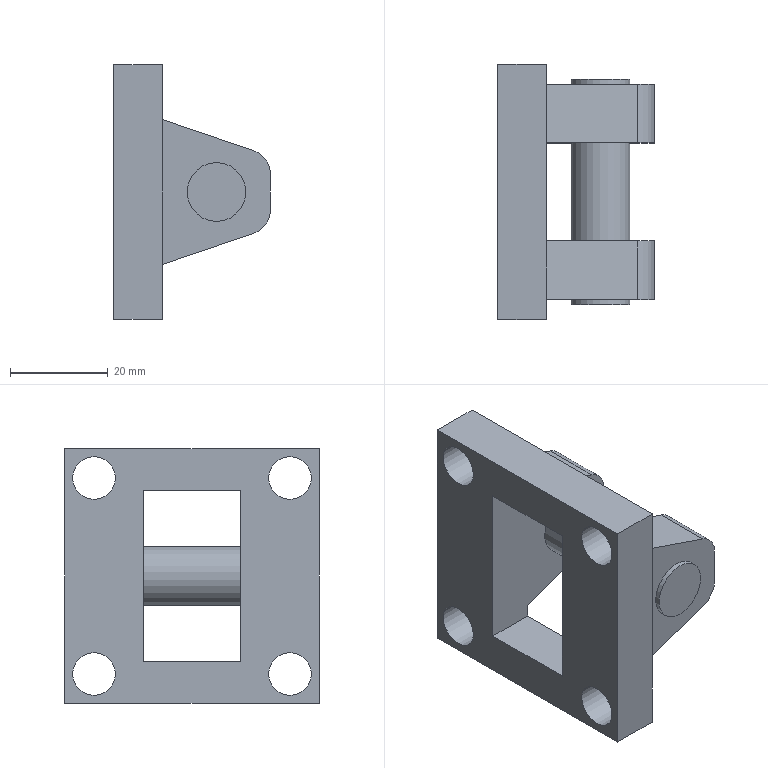Part | STEP file | 冲床-300配套压波_id670_x_t | 1 solid | 31 faces | box 32 x 52 x 52 mm | volume 31697 mm3 | plane 20 | cylinder 11 | commonest cylinder face diameters 8.7 x4 10 x4 12 x3
STEP:
#1=CARTESIAN_POINT('',(1965.,-26.,-387.));
#2=VERTEX_POINT('',#1);
#3=CARTESIAN_POINT('',(1965.,26.,-387.));
#4=VERTEX_POINT('',#3);
#5=CARTESIAN_POINT('',(1965.,-26.,-387.));
#6=DIRECTION('',(0.,1.,0.));
#7=VECTOR('',#6,1.);
#8=LINE('',#5,#7);
#9=EDGE_CURVE('',#2,#4,#8,.T.);
#10=ORIENTED_EDGE('',*,*,#9,.T.);
#11=CARTESIAN_POINT('',(1965.,26.,-335.));
#12=VERTEX_POINT('',#11);
#13=CARTESIAN_POINT('',(1965.,26.,-387.));
#14=DIRECTION('',(0.,0.,1.));
#15=VECTOR('',#14,1.);
#16=LINE('',#13,#15);
#17=EDGE_CURVE('',#4,#12,#16,.T.);
#18=ORIENTED_EDGE('',*,*,#17,.T.);
#19=CARTESIAN_POINT('',(1965.,-26.,-335.));
#20=VERTEX_POINT('',#19);
#21=CARTESIAN_POINT('',(1965.,26.,-335.));
#22=DIRECTION('',(0.,-1.,0.));
#23=VECTOR('',#22,1.);
#24=LINE('',#21,#23);
#25=EDGE_CURVE('',#12,#20,#24,.T.);
#26=ORIENTED_EDGE('',*,*,#25,.T.);
#27=CARTESIAN_POINT('',(1965.,-26.,-335.));
#28=DIRECTION('',(0.,0.,-1.));
#29=VECTOR('',#28,1.);
#30=LINE('',#27,#29);
#31=EDGE_CURVE('',#20,#2,#30,.T.);
#32=ORIENTED_EDGE('',*,*,#31,.T.);
#33=EDGE_LOOP('',(#10,#18,#26,#32));
#34=FACE_BOUND('',#33,.T.);
#35=CARTESIAN_POINT('',(1965.,-20.,-385.35));
#36=VERTEX_POINT('',#35);
#37=CARTESIAN_POINT('',(1965.,-20.,-381.));
#38=DIRECTION('',(1.,0.,0.));
#39=DIRECTION('',(0.,0.,-1.));
#40=AXIS2_PLACEMENT_3D('',#37,#38,#39);
#41=CIRCLE('',#40,4.35);
#42=EDGE_CURVE('',#36,#36,#41,.T.);
#43=ORIENTED_EDGE('',*,*,#42,.F.);
#44=EDGE_LOOP('',(#43));
#45=FACE_BOUND('',#44,.T.);
#46=CARTESIAN_POINT('',(1965.,-20.,-345.35));
#47=VERTEX_POINT('',#46);
#48=CARTESIAN_POINT('',(1965.,-20.,-341.));
#49=DIRECTION('',(1.,0.,0.));
#50=DIRECTION('',(0.,0.,-1.));
#51=AXIS2_PLACEMENT_3D('',#48,#49,#50);
#52=CIRCLE('',#51,4.35);
#53=EDGE_CURVE('',#47,#47,#52,.T.);
#54=ORIENTED_EDGE('',*,*,#53,.F.);
#55=EDGE_LOOP('',(#54));
#56=FACE_BOUND('',#55,.T.);
#57=CARTESIAN_POINT('',(1965.,20.,-385.35));
#58=VERTEX_POINT('',#57);
#59=CARTESIAN_POINT('',(1965.,20.,-381.));
#60=DIRECTION('',(1.,0.,0.));
#61=DIRECTION('',(0.,0.,-1.));
#62=AXIS2_PLACEMENT_3D('',#59,#60,#61);
#63=CIRCLE('',#62,4.35);
#64=EDGE_CURVE('',#58,#58,#63,.T.);
#65=ORIENTED_EDGE('',*,*,#64,.F.);
#66=EDGE_LOOP('',(#65));
#67=FACE_BOUND('',#66,.T.);
#68=CARTESIAN_POINT('',(1965.,20.,-345.35));
#69=VERTEX_POINT('',#68);
#70=CARTESIAN_POINT('',(1965.,20.,-341.));
#71=DIRECTION('',(1.,0.,0.));
#72=DIRECTION('',(0.,0.,-1.));
#73=AXIS2_PLACEMENT_3D('',#70,#71,#72);
#74=CIRCLE('',#73,4.35);
#75=EDGE_CURVE('',#69,#69,#74,.T.);
#76=ORIENTED_EDGE('',*,*,#75,.F.);
#77=EDGE_LOOP('',(#76));
#78=FACE_BOUND('',#77,.T.);
#79=CARTESIAN_POINT('',(1965.,10.,-343.5));
#80=VERTEX_POINT('',#79);
#81=CARTESIAN_POINT('',(1965.,10.,-346.208));
#82=VERTEX_POINT('',#81);
#83=CARTESIAN_POINT('',(1965.,10.,-343.5));
#84=DIRECTION('',(0.,0.,-1.));
#85=VECTOR('',#84,1.);
#86=LINE('',#83,#85);
#87=EDGE_CURVE('',#80,#82,#86,.T.);
#88=ORIENTED_EDGE('',*,*,#87,.T.);
#89=CARTESIAN_POINT('',(1965.,22.,-346.208));
#90=VERTEX_POINT('',#89);
#91=CARTESIAN_POINT('',(1965.,10.,-346.208));
#92=DIRECTION('',(0.,1.,0.));
#93=VECTOR('',#92,1.);
#94=LINE('',#91,#93);
#95=EDGE_CURVE('',#82,#90,#94,.T.);
#96=ORIENTED_EDGE('',*,*,#95,.T.);
#97=CARTESIAN_POINT('',(1965.,22.,-375.792));
#98=VERTEX_POINT('',#97);
#99=CARTESIAN_POINT('',(1965.,22.,-381.));
#100=DIRECTION('',(0.,0.,-1.));
#101=VECTOR('',#100,1.);
#102=LINE('',#99,#101);
#103=EDGE_CURVE('',#90,#98,#102,.T.);
#104=ORIENTED_EDGE('',*,*,#103,.T.);
#105=CARTESIAN_POINT('',(1965.,10.,-375.792));
#106=VERTEX_POINT('',#105);
#107=CARTESIAN_POINT('',(1965.,22.,-375.792));
#108=DIRECTION('',(0.,-1.,0.));
#109=VECTOR('',#108,1.);
#110=LINE('',#107,#109);
#111=EDGE_CURVE('',#98,#106,#110,.T.);
#112=ORIENTED_EDGE('',*,*,#111,.T.);
#113=CARTESIAN_POINT('',(1965.,10.,-378.5));
#114=VERTEX_POINT('',#113);
#115=CARTESIAN_POINT('',(1965.,10.,-343.5));
#116=DIRECTION('',(0.,0.,-1.));
#117=VECTOR('',#116,1.);
#118=LINE('',#115,#117);
#119=EDGE_CURVE('',#106,#114,#118,.T.);
#120=ORIENTED_EDGE('',*,*,#119,.T.);
#121=CARTESIAN_POINT('',(1965.,-10.,-378.5));
#122=VERTEX_POINT('',#121);
#123=CARTESIAN_POINT('',(1965.,10.,-378.5));
#124=DIRECTION('',(0.,-1.,0.));
#125=VECTOR('',#124,1.);
#126=LINE('',#123,#125);
#127=EDGE_CURVE('',#114,#122,#126,.T.);
#128=ORIENTED_EDGE('',*,*,#127,.T.);
#129=CARTESIAN_POINT('',(1965.,-10.,-375.792));
#130=VERTEX_POINT('',#129);
#131=CARTESIAN_POINT('',(1965.,-10.,-378.5));
#132=DIRECTION('',(0.,0.,1.));
#133=VECTOR('',#132,1.);
#134=LINE('',#131,#133);
#135=EDGE_CURVE('',#122,#130,#134,.T.);
#136=ORIENTED_EDGE('',*,*,#135,.T.);
#137=CARTESIAN_POINT('',(1965.,-22.,-375.792));
#138=VERTEX_POINT('',#137);
#139=CARTESIAN_POINT('',(1965.,-20.,-375.792));
#140=DIRECTION('',(0.,-1.,0.));
#141=VECTOR('',#140,1.);
#142=LINE('',#139,#141);
#143=EDGE_CURVE('',#130,#138,#142,.T.);
#144=ORIENTED_EDGE('',*,*,#143,.T.);
#145=CARTESIAN_POINT('',(1965.,-22.,-346.208));
#146=VERTEX_POINT('',#145);
#147=CARTESIAN_POINT('',(1965.,-22.,-381.));
#148=DIRECTION('',(0.,0.,1.));
#149=VECTOR('',#148,1.);
#150=LINE('',#147,#149);
#151=EDGE_CURVE('',#138,#146,#150,.T.);
#152=ORIENTED_EDGE('',*,*,#151,.T.);
#153=CARTESIAN_POINT('',(1965.,-10.,-346.208));
#154=VERTEX_POINT('',#153);
#155=CARTESIAN_POINT('',(1965.,-20.,-346.208));
#156=DIRECTION('',(0.,1.,0.));
#157=VECTOR('',#156,1.);
#158=LINE('',#155,#157);
#159=EDGE_CURVE('',#146,#154,#158,.T.);
#160=ORIENTED_EDGE('',*,*,#159,.T.);
#161=CARTESIAN_POINT('',(1965.,-10.,-343.5));
#162=VERTEX_POINT('',#161);
#163=CARTESIAN_POINT('',(1965.,-10.,-378.5));
#164=DIRECTION('',(0.,0.,1.));
#165=VECTOR('',#164,1.);
#166=LINE('',#163,#165);
#167=EDGE_CURVE('',#154,#162,#166,.T.);
#168=ORIENTED_EDGE('',*,*,#167,.T.);
#169=CARTESIAN_POINT('',(1965.,-10.,-343.5));
#170=DIRECTION('',(0.,1.,0.));
#171=VECTOR('',#170,1.);
#172=LINE('',#169,#171);
#173=EDGE_CURVE('',#162,#80,#172,.T.);
#174=ORIENTED_EDGE('',*,*,#173,.T.);
#175=EDGE_LOOP('',(#88,#96,#104,#112,#120,#128,#136,#144,#152,#160,#168,#174));
#176=FACE_BOUND('',#175,.T.);
#177=CARTESIAN_POINT('',(1965.,-20.,-381.));
#178=DIRECTION('',(1.,0.,0.));
#179=DIRECTION('',(0.,0.,-1.));
#180=AXIS2_PLACEMENT_3D('',#177,#178,#179);
#181=PLANE('',#180);
#182=ADVANCED_FACE('',(#34,#45,#56,#67,#78,#176),#181,.T.);
#183=CARTESIAN_POINT('',(1976.,-10.,-355.));
#184=VERTEX_POINT('',#183);
#185=CARTESIAN_POINT('',(1976.,-10.,-361.));
#186=DIRECTION('',(0.,1.,0.));
#187=DIRECTION('',(0.,0.,1.));
#188=AXIS2_PLACEMENT_3D('',#185,#186,#187);
#189=CIRCLE('',#188,6.);
#190=EDGE_CURVE('',#184,#184,#189,.T.);
#191=ORIENTED_EDGE('',*,*,#190,.F.);
#192=EDGE_LOOP('',(#191));
#193=FACE_BOUND('',#192,.T.);
#194=CARTESIAN_POINT('',(1983.613,-10.,-352.554));
#195=VERTEX_POINT('',#194);
#196=CARTESIAN_POINT('',(1965.903,-10.,-346.516));
#197=DIRECTION('',(0.9465,0.,-0.3227));
#198=VECTOR('',#197,1.);
#199=LINE('',#196,#198);
#200=EDGE_CURVE('',#154,#195,#199,.T.);
#201=ORIENTED_EDGE('',*,*,#200,.T.);
#202=CARTESIAN_POINT('',(1987.,-10.,-357.286));
#203=VERTEX_POINT('',#202);
#204=CARTESIAN_POINT('',(1982.,-10.,-357.286));
#205=DIRECTION('',(0.,1.,0.));
#206=DIRECTION('',(0.,0.,1.));
#207=AXIS2_PLACEMENT_3D('',#204,#205,#206);
#208=CIRCLE('',#207,5.);
#209=EDGE_CURVE('',#195,#203,#208,.T.);
#210=ORIENTED_EDGE('',*,*,#209,.T.);
#211=CARTESIAN_POINT('',(1987.,-10.,-364.714));
#212=VERTEX_POINT('',#211);
#213=CARTESIAN_POINT('',(1987.,-10.,-346.208));
#214=DIRECTION('',(0.,0.,-1.));
#215=VECTOR('',#214,1.);
#216=LINE('',#213,#215);
#217=EDGE_CURVE('',#203,#212,#216,.T.);
#218=ORIENTED_EDGE('',*,*,#217,.T.);
#219=CARTESIAN_POINT('',(1983.613,-10.,-369.446));
#220=VERTEX_POINT('',#219);
#221=CARTESIAN_POINT('',(1982.,-10.,-364.714));
#222=DIRECTION('',(0.,1.,0.));
#223=DIRECTION('',(0.,0.,1.));
#224=AXIS2_PLACEMENT_3D('',#221,#222,#223);
#225=CIRCLE('',#224,5.);
#226=EDGE_CURVE('',#212,#220,#225,.T.);
#227=ORIENTED_EDGE('',*,*,#226,.T.);
#228=CARTESIAN_POINT('',(1955.214,-10.,-379.128));
#229=DIRECTION('',(-0.9465,0.,-0.3227));
#230=VECTOR('',#229,1.);
#231=LINE('',#228,#230);
#232=EDGE_CURVE('',#220,#130,#231,.T.);
#233=ORIENTED_EDGE('',*,*,#232,.T.);
#234=ORIENTED_EDGE('',*,*,#135,.F.);
#235=CARTESIAN_POINT('',(1955.,-10.,-378.5));
#236=VERTEX_POINT('',#235);
#237=CARTESIAN_POINT('',(1955.,-10.,-378.5));
#238=DIRECTION('',(1.,0.,0.));
#239=VECTOR('',#238,1.);
#240=LINE('',#237,#239);
#241=EDGE_CURVE('',#236,#122,#240,.T.);
#242=ORIENTED_EDGE('',*,*,#241,.F.);
#243=CARTESIAN_POINT('',(1955.,-10.,-343.5));
#244=VERTEX_POINT('',#243);
#245=CARTESIAN_POINT('',(1955.,-10.,-378.5));
#246=DIRECTION('',(0.,0.,1.));
#247=VECTOR('',#246,1.);
#248=LINE('',#245,#247);
#249=EDGE_CURVE('',#236,#244,#248,.T.);
#250=ORIENTED_EDGE('',*,*,#249,.T.);
#251=CARTESIAN_POINT('',(1955.,-10.,-343.5));
#252=DIRECTION('',(1.,0.,0.));
#253=VECTOR('',#252,1.);
#254=LINE('',#251,#253);
#255=EDGE_CURVE('',#244,#162,#254,.T.);
#256=ORIENTED_EDGE('',*,*,#255,.T.);
#257=ORIENTED_EDGE('',*,*,#167,.F.);
#258=EDGE_LOOP('',(#201,#210,#218,#227,#233,#234,#242,#250,#256,#257));
#259=FACE_BOUND('',#258,.T.);
#260=CARTESIAN_POINT('',(1955.,-10.,-378.5));
#261=DIRECTION('',(0.,1.,0.));
#262=DIRECTION('',(0.,0.,1.));
#263=AXIS2_PLACEMENT_3D('',#260,#261,#262);
#264=PLANE('',#263);
#265=ADVANCED_FACE('',(#193,#259),#264,.T.);
#266=ORIENTED_EDGE('',*,*,#173,.F.);
#267=ORIENTED_EDGE('',*,*,#255,.F.);
#268=CARTESIAN_POINT('',(1955.,10.,-343.5));
#269=VERTEX_POINT('',#268);
#270=CARTESIAN_POINT('',(1955.,-10.,-343.5));
#271=DIRECTION('',(0.,1.,0.));
#272=VECTOR('',#271,1.);
#273=LINE('',#270,#272);
#274=EDGE_CURVE('',#244,#269,#273,.T.);
#275=ORIENTED_EDGE('',*,*,#274,.T.);
#276=CARTESIAN_POINT('',(1955.,10.,-343.5));
#277=DIRECTION('',(1.,0.,0.));
#278=VECTOR('',#277,1.);
#279=LINE('',#276,#278);
#280=EDGE_CURVE('',#269,#80,#279,.T.);
#281=ORIENTED_EDGE('',*,*,#280,.T.);
#282=EDGE_LOOP('',(#266,#267,#275,#281));
#283=FACE_OUTER_BOUND('',#282,.T.);
#284=CARTESIAN_POINT('',(1955.,-10.,-343.5));
#285=DIRECTION('',(0.,0.,-1.));
#286=DIRECTION('',(0.,1.,0.));
#287=AXIS2_PLACEMENT_3D('',#284,#285,#286);
#288=PLANE('',#287);
#289=ADVANCED_FACE('',(#283),#288,.T.);
#290=CARTESIAN_POINT('',(1976.,10.,-367.));
#291=VERTEX_POINT('',#290);
#292=CARTESIAN_POINT('',(1976.,10.,-361.));
#293=DIRECTION('',(0.,-1.,0.));
#294=DIRECTION('',(0.,0.,-1.));
#295=AXIS2_PLACEMENT_3D('',#292,#293,#294);
#296=CIRCLE('',#295,6.);
#297=EDGE_CURVE('',#291,#291,#296,.T.);
#298=ORIENTED_EDGE('',*,*,#297,.F.);
#299=EDGE_LOOP('',(#298));
#300=FACE_BOUND('',#299,.T.);
#301=CARTESIAN_POINT('',(1983.613,10.,-369.446));
#302=VERTEX_POINT('',#301);
#303=CARTESIAN_POINT('',(1965.,10.,-375.792));
#304=DIRECTION('',(0.9465,0.,0.3227));
#305=VECTOR('',#304,1.);
#306=LINE('',#303,#305);
#307=EDGE_CURVE('',#106,#302,#306,.T.);
#308=ORIENTED_EDGE('',*,*,#307,.T.);
#309=CARTESIAN_POINT('',(1987.,10.,-364.714));
#310=VERTEX_POINT('',#309);
#311=CARTESIAN_POINT('',(1982.,10.,-364.714));
#312=DIRECTION('',(0.,-1.,0.));
#313=DIRECTION('',(0.,0.,-1.));
#314=AXIS2_PLACEMENT_3D('',#311,#312,#313);
#315=CIRCLE('',#314,5.);
#316=EDGE_CURVE('',#302,#310,#315,.T.);
#317=ORIENTED_EDGE('',*,*,#316,.T.);
#318=CARTESIAN_POINT('',(1987.,10.,-357.286));
#319=VERTEX_POINT('',#318);
#320=CARTESIAN_POINT('',(1987.,10.,-375.792));
#321=DIRECTION('',(0.,0.,1.));
#322=VECTOR('',#321,1.);
#323=LINE('',#320,#322);
#324=EDGE_CURVE('',#310,#319,#323,.T.);
#325=ORIENTED_EDGE('',*,*,#324,.T.);
#326=CARTESIAN_POINT('',(1983.613,10.,-352.554));
#327=VERTEX_POINT('',#326);
#328=CARTESIAN_POINT('',(1982.,10.,-357.286));
#329=DIRECTION('',(0.,-1.,0.));
#330=DIRECTION('',(0.,0.,-1.));
#331=AXIS2_PLACEMENT_3D('',#328,#329,#330);
#332=CIRCLE('',#331,5.);
#333=EDGE_CURVE('',#319,#327,#332,.T.);
#334=ORIENTED_EDGE('',*,*,#333,.T.);
#335=CARTESIAN_POINT('',(1965.,10.,-346.208));
#336=DIRECTION('',(-0.9465,0.,0.3227));
#337=VECTOR('',#336,1.);
#338=LINE('',#335,#337);
#339=EDGE_CURVE('',#327,#82,#338,.T.);
#340=ORIENTED_EDGE('',*,*,#339,.T.);
#341=ORIENTED_EDGE('',*,*,#87,.F.);
#342=ORIENTED_EDGE('',*,*,#280,.F.);
#343=CARTESIAN_POINT('',(1955.,10.,-378.5));
#344=VERTEX_POINT('',#343);
#345=CARTESIAN_POINT('',(1955.,10.,-343.5));
#346=DIRECTION('',(0.,0.,-1.));
#347=VECTOR('',#346,1.);
#348=LINE('',#345,#347);
#349=EDGE_CURVE('',#269,#344,#348,.T.);
#350=ORIENTED_EDGE('',*,*,#349,.T.);
#351=CARTESIAN_POINT('',(1955.,10.,-378.5));
#352=DIRECTION('',(1.,0.,0.));
#353=VECTOR('',#352,1.);
#354=LINE('',#351,#353);
#355=EDGE_CURVE('',#344,#114,#354,.T.);
#356=ORIENTED_EDGE('',*,*,#355,.T.);
#357=ORIENTED_EDGE('',*,*,#119,.F.);
#358=EDGE_LOOP('',(#308,#317,#325,#334,#340,#341,#342,#350,#356,#357));
#359=FACE_BOUND('',#358,.T.);
#360=CARTESIAN_POINT('',(1955.,10.,-343.5));
#361=DIRECTION('',(0.,-1.,0.));
#362=DIRECTION('',(0.,0.,-1.));
#363=AXIS2_PLACEMENT_3D('',#360,#361,#362);
#364=PLANE('',#363);
#365=ADVANCED_FACE('',(#300,#359),#364,.T.);
#366=ORIENTED_EDGE('',*,*,#9,.F.);
#367=CARTESIAN_POINT('',(1955.,-26.,-387.));
#368=VERTEX_POINT('',#367);
#369=CARTESIAN_POINT('',(1955.,-26.,-387.));
#370=DIRECTION('',(1.,0.,0.));
#371=VECTOR('',#370,1.);
#372=LINE('',#369,#371);
#373=EDGE_CURVE('',#368,#2,#372,.T.);
#374=ORIENTED_EDGE('',*,*,#373,.F.);
#375=CARTESIAN_POINT('',(1955.,26.,-387.));
#376=VERTEX_POINT('',#375);
#377=CARTESIAN_POINT('',(1955.,-26.,-387.));
#378=DIRECTION('',(0.,1.,0.));
#379=VECTOR('',#378,1.);
#380=LINE('',#377,#379);
#381=EDGE_CURVE('',#368,#376,#380,.T.);
#382=ORIENTED_EDGE('',*,*,#381,.T.);
#383=CARTESIAN_POINT('',(1955.,26.,-387.));
#384=DIRECTION('',(1.,0.,0.));
#385=VECTOR('',#384,1.);
#386=LINE('',#383,#385);
#387=EDGE_CURVE('',#376,#4,#386,.T.);
#388=ORIENTED_EDGE('',*,*,#387,.T.);
#389=EDGE_LOOP('',(#366,#374,#382,#388));
#390=FACE_OUTER_BOUND('',#389,.T.);
#391=CARTESIAN_POINT('',(1955.,-26.,-387.));
#392=DIRECTION('',(0.,0.,-1.));
#393=DIRECTION('',(-1.,0.,0.));
#394=AXIS2_PLACEMENT_3D('',#391,#392,#393);
#395=PLANE('',#394);
#396=ADVANCED_FACE('',(#390),#395,.T.);
#397=ORIENTED_EDGE('',*,*,#17,.F.);
#398=ORIENTED_EDGE('',*,*,#387,.F.);
#399=CARTESIAN_POINT('',(1955.,26.,-335.));
#400=VERTEX_POINT('',#399);
#401=CARTESIAN_POINT('',(1955.,26.,-387.));
#402=DIRECTION('',(0.,0.,1.));
#403=VECTOR('',#402,1.);
#404=LINE('',#401,#403);
#405=EDGE_CURVE('',#376,#400,#404,.T.);
#406=ORIENTED_EDGE('',*,*,#405,.T.);
#407=CARTESIAN_POINT('',(1955.,26.,-335.));
#408=DIRECTION('',(1.,0.,0.));
#409=VECTOR('',#408,1.);
#410=LINE('',#407,#409);
#411=EDGE_CURVE('',#400,#12,#410,.T.);
#412=ORIENTED_EDGE('',*,*,#411,.T.);
#413=EDGE_LOOP('',(#397,#398,#406,#412));
#414=FACE_OUTER_BOUND('',#413,.T.);
#415=CARTESIAN_POINT('',(1955.,26.,-387.));
#416=DIRECTION('',(0.,1.,0.));
#417=DIRECTION('',(0.,0.,1.));
#418=AXIS2_PLACEMENT_3D('',#415,#416,#417);
#419=PLANE('',#418);
#420=ADVANCED_FACE('',(#414),#419,.T.);
#421=ORIENTED_EDGE('',*,*,#25,.F.);
#422=ORIENTED_EDGE('',*,*,#411,.F.);
#423=CARTESIAN_POINT('',(1955.,-26.,-335.));
#424=VERTEX_POINT('',#423);
#425=CARTESIAN_POINT('',(1955.,26.,-335.));
#426=DIRECTION('',(0.,-1.,0.));
#427=VECTOR('',#426,1.);
#428=LINE('',#425,#427);
#429=EDGE_CURVE('',#400,#424,#428,.T.);
#430=ORIENTED_EDGE('',*,*,#429,.T.);
#431=CARTESIAN_POINT('',(1955.,-26.,-335.));
#432=DIRECTION('',(1.,0.,0.));
#433=VECTOR('',#432,1.);
#434=LINE('',#431,#433);
#435=EDGE_CURVE('',#424,#20,#434,.T.);
#436=ORIENTED_EDGE('',*,*,#435,.T.);
#437=EDGE_LOOP('',(#421,#422,#430,#436));
#438=FACE_OUTER_BOUND('',#437,.T.);
#439=CARTESIAN_POINT('',(1955.,26.,-335.));
#440=DIRECTION('',(0.,0.,1.));
#441=DIRECTION('',(1.,0.,0.));
#442=AXIS2_PLACEMENT_3D('',#439,#440,#441);
#443=PLANE('',#442);
#444=ADVANCED_FACE('',(#438),#443,.T.);
#445=CARTESIAN_POINT('',(1955.,20.,-345.35));
#446=VERTEX_POINT('',#445);
#447=CARTESIAN_POINT('',(1955.,20.,-341.));
#448=DIRECTION('',(1.,0.,0.));
#449=DIRECTION('',(0.,0.,-1.));
#450=AXIS2_PLACEMENT_3D('',#447,#448,#449);
#451=CIRCLE('',#450,4.35);
#452=EDGE_CURVE('',#446,#446,#451,.T.);
#453=ORIENTED_EDGE('',*,*,#452,.F.);
#454=EDGE_LOOP('',(#453));
#455=FACE_BOUND('',#454,.T.);
#456=ORIENTED_EDGE('',*,*,#75,.T.);
#457=EDGE_LOOP('',(#456));
#458=FACE_BOUND('',#457,.T.);
#459=CARTESIAN_POINT('',(1955.,20.,-341.));
#460=DIRECTION('',(1.,0.,0.));
#461=DIRECTION('',(0.,0.,-1.));
#462=AXIS2_PLACEMENT_3D('',#459,#460,#461);
#463=CYLINDRICAL_SURFACE('',#462,4.35);
#464=ADVANCED_FACE('',(#455,#458),#463,.F.);
#465=CARTESIAN_POINT('',(1955.,20.,-385.35));
#466=VERTEX_POINT('',#465);
#467=CARTESIAN_POINT('',(1955.,20.,-381.));
#468=DIRECTION('',(1.,0.,0.));
#469=DIRECTION('',(0.,0.,-1.));
#470=AXIS2_PLACEMENT_3D('',#467,#468,#469);
#471=CIRCLE('',#470,4.35);
#472=EDGE_CURVE('',#466,#466,#471,.T.);
#473=ORIENTED_EDGE('',*,*,#472,.F.);
#474=EDGE_LOOP('',(#473));
#475=FACE_BOUND('',#474,.T.);
#476=ORIENTED_EDGE('',*,*,#64,.T.);
#477=EDGE_LOOP('',(#476));
#478=FACE_BOUND('',#477,.T.);
#479=CARTESIAN_POINT('',(1955.,20.,-381.));
#480=DIRECTION('',(1.,0.,0.));
#481=DIRECTION('',(0.,0.,-1.));
#482=AXIS2_PLACEMENT_3D('',#479,#480,#481);
#483=CYLINDRICAL_SURFACE('',#482,4.35);
#484=ADVANCED_FACE('',(#475,#478),#483,.F.);
#485=CARTESIAN_POINT('',(1955.,-20.,-345.35));
#486=VERTEX_POINT('',#485);
#487=CARTESIAN_POINT('',(1955.,-20.,-341.));
#488=DIRECTION('',(1.,0.,0.));
#489=DIRECTION('',(0.,0.,-1.));
#490=AXIS2_PLACEMENT_3D('',#487,#488,#489);
#491=CIRCLE('',#490,4.35);
#492=EDGE_CURVE('',#486,#486,#491,.T.);
#493=ORIENTED_EDGE('',*,*,#492,.F.);
#494=EDGE_LOOP('',(#493));
#495=FACE_BOUND('',#494,.T.);
#496=ORIENTED_EDGE('',*,*,#53,.T.);
#497=EDGE_LOOP('',(#496));
#498=FACE_BOUND('',#497,.T.);
#499=CARTESIAN_POINT('',(1955.,-20.,-341.));
#500=DIRECTION('',(1.,0.,0.));
#501=DIRECTION('',(0.,0.,-1.));
#502=AXIS2_PLACEMENT_3D('',#499,#500,#501);
#503=CYLINDRICAL_SURFACE('',#502,4.35);
#504=ADVANCED_FACE('',(#495,#498),#503,.F.);
#505=CARTESIAN_POINT('',(1955.,-20.,-385.35));
#506=VERTEX_POINT('',#505);
#507=CARTESIAN_POINT('',(1955.,-20.,-381.));
#508=DIRECTION('',(1.,0.,0.));
#509=DIRECTION('',(0.,0.,-1.));
#510=AXIS2_PLACEMENT_3D('',#507,#508,#509);
#511=CIRCLE('',#510,4.35);
#512=EDGE_CURVE('',#506,#506,#511,.T.);
#513=ORIENTED_EDGE('',*,*,#512,.F.);
#514=EDGE_LOOP('',(#513));
#515=FACE_BOUND('',#514,.T.);
#516=ORIENTED_EDGE('',*,*,#42,.T.);
#517=EDGE_LOOP('',(#516));
#518=FACE_BOUND('',#517,.T.);
#519=CARTESIAN_POINT('',(1955.,-20.,-381.));
#520=DIRECTION('',(1.,0.,0.));
#521=DIRECTION('',(0.,0.,-1.));
#522=AXIS2_PLACEMENT_3D('',#519,#520,#521);
#523=CYLINDRICAL_SURFACE('',#522,4.35);
#524=ADVANCED_FACE('',(#515,#518),#523,.F.);
#525=ORIENTED_EDGE('',*,*,#31,.F.);
#526=ORIENTED_EDGE('',*,*,#435,.F.);
#527=CARTESIAN_POINT('',(1955.,-26.,-335.));
#528=DIRECTION('',(0.,0.,-1.));
#529=VECTOR('',#528,1.);
#530=LINE('',#527,#529);
#531=EDGE_CURVE('',#424,#368,#530,.T.);
#532=ORIENTED_EDGE('',*,*,#531,.T.);
#533=ORIENTED_EDGE('',*,*,#373,.T.);
#534=EDGE_LOOP('',(#525,#526,#532,#533));
#535=FACE_OUTER_BOUND('',#534,.T.);
#536=CARTESIAN_POINT('',(1955.,-26.,-335.));
#537=DIRECTION('',(0.,-1.,0.));
#538=DIRECTION('',(0.,0.,-1.));
#539=AXIS2_PLACEMENT_3D('',#536,#537,#538);
#540=PLANE('',#539);
#541=ADVANCED_FACE('',(#535),#540,.T.);
#542=ORIENTED_EDGE('',*,*,#127,.F.);
#543=ORIENTED_EDGE('',*,*,#355,.F.);
#544=CARTESIAN_POINT('',(1955.,10.,-378.5));
#545=DIRECTION('',(0.,-1.,0.));
#546=VECTOR('',#545,1.);
#547=LINE('',#544,#546);
#548=EDGE_CURVE('',#344,#236,#547,.T.);
#549=ORIENTED_EDGE('',*,*,#548,.T.);
#550=ORIENTED_EDGE('',*,*,#241,.T.);
#551=EDGE_LOOP('',(#542,#543,#549,#550));
#552=FACE_OUTER_BOUND('',#551,.T.);
#553=CARTESIAN_POINT('',(1955.,10.,-378.5));
#554=DIRECTION('',(0.,0.,1.));
#555=DIRECTION('',(0.,-1.,0.));
#556=AXIS2_PLACEMENT_3D('',#553,#554,#555);
#557=PLANE('',#556);
#558=ADVANCED_FACE('',(#552),#557,.T.);
#559=ORIENTED_EDGE('',*,*,#548,.F.);
#560=ORIENTED_EDGE('',*,*,#349,.F.);
#561=ORIENTED_EDGE('',*,*,#274,.F.);
#562=ORIENTED_EDGE('',*,*,#249,.F.);
#563=EDGE_LOOP('',(#559,#560,#561,#562));
#564=FACE_BOUND('',#563,.T.);
#565=ORIENTED_EDGE('',*,*,#381,.F.);
#566=ORIENTED_EDGE('',*,*,#531,.F.);
#567=ORIENTED_EDGE('',*,*,#429,.F.);
#568=ORIENTED_EDGE('',*,*,#405,.F.);
#569=EDGE_LOOP('',(#565,#566,#567,#568));
#570=FACE_BOUND('',#569,.T.);
#571=ORIENTED_EDGE('',*,*,#512,.T.);
#572=EDGE_LOOP('',(#571));
#573=FACE_BOUND('',#572,.T.);
#574=ORIENTED_EDGE('',*,*,#492,.T.);
#575=EDGE_LOOP('',(#574));
#576=FACE_BOUND('',#575,.T.);
#577=ORIENTED_EDGE('',*,*,#472,.T.);
#578=EDGE_LOOP('',(#577));
#579=FACE_BOUND('',#578,.T.);
#580=ORIENTED_EDGE('',*,*,#452,.T.);
#581=EDGE_LOOP('',(#580));
#582=FACE_BOUND('',#581,.T.);
#583=CARTESIAN_POINT('',(1955.,-20.,-381.));
#584=DIRECTION('',(1.,0.,0.));
#585=DIRECTION('',(0.,0.,-1.));
#586=AXIS2_PLACEMENT_3D('',#583,#584,#585);
#587=PLANE('',#586);
#588=ADVANCED_FACE('',(#564,#570,#573,#576,#579,#582),#587,.F.);
#589=CARTESIAN_POINT('',(1976.,-22.,-355.));
#590=VERTEX_POINT('',#589);
#591=CARTESIAN_POINT('',(1976.,-22.,-361.));
#592=DIRECTION('',(0.,1.,0.));
#593=DIRECTION('',(0.,0.,1.));
#594=AXIS2_PLACEMENT_3D('',#591,#592,#593);
#595=CIRCLE('',#594,6.);
#596=EDGE_CURVE('',#590,#590,#595,.T.);
#597=ORIENTED_EDGE('',*,*,#596,.T.);
#598=EDGE_LOOP('',(#597));
#599=FACE_BOUND('',#598,.T.);
#600=CARTESIAN_POINT('',(1987.,-22.,-364.714));
#601=VERTEX_POINT('',#600);
#602=CARTESIAN_POINT('',(1987.,-22.,-357.286));
#603=VERTEX_POINT('',#602);
#604=CARTESIAN_POINT('',(1987.,-22.,-375.792));
#605=DIRECTION('',(0.,0.,1.));
#606=VECTOR('',#605,1.);
#607=LINE('',#604,#606);
#608=EDGE_CURVE('',#601,#603,#607,.T.);
#609=ORIENTED_EDGE('',*,*,#608,.T.);
#610=CARTESIAN_POINT('',(1983.613,-22.,-352.554));
#611=VERTEX_POINT('',#610);
#612=CARTESIAN_POINT('',(1982.,-22.,-357.286));
#613=DIRECTION('',(0.,-1.,0.));
#614=DIRECTION('',(0.,0.,1.));
#615=AXIS2_PLACEMENT_3D('',#612,#613,#614);
#616=CIRCLE('',#615,5.);
#617=EDGE_CURVE('',#603,#611,#616,.T.);
#618=ORIENTED_EDGE('',*,*,#617,.T.);
#619=CARTESIAN_POINT('',(1965.076,-22.,-346.234));
#620=DIRECTION('',(-0.9465,0.,0.3227));
#621=VECTOR('',#620,1.);
#622=LINE('',#619,#621);
#623=EDGE_CURVE('',#611,#146,#622,.T.);
#624=ORIENTED_EDGE('',*,*,#623,.T.);
#625=ORIENTED_EDGE('',*,*,#151,.F.);
#626=CARTESIAN_POINT('',(1983.613,-22.,-369.446));
#627=VERTEX_POINT('',#626);
#628=CARTESIAN_POINT('',(1956.041,-22.,-378.846));
#629=DIRECTION('',(0.9465,0.,0.3227));
#630=VECTOR('',#629,1.);
#631=LINE('',#628,#630);
#632=EDGE_CURVE('',#138,#627,#631,.T.);
#633=ORIENTED_EDGE('',*,*,#632,.T.);
#634=CARTESIAN_POINT('',(1982.,-22.,-364.714));
#635=DIRECTION('',(0.,-1.,0.));
#636=DIRECTION('',(0.,0.,1.));
#637=AXIS2_PLACEMENT_3D('',#634,#635,#636);
#638=CIRCLE('',#637,5.);
#639=EDGE_CURVE('',#627,#601,#638,.T.);
#640=ORIENTED_EDGE('',*,*,#639,.T.);
#641=EDGE_LOOP('',(#609,#618,#624,#625,#633,#640));
#642=FACE_BOUND('',#641,.T.);
#643=CARTESIAN_POINT('',(1955.,-22.,-375.792));
#644=DIRECTION('',(0.,1.,0.));
#645=DIRECTION('',(0.,0.,1.));
#646=AXIS2_PLACEMENT_3D('',#643,#644,#645);
#647=PLANE('',#646);
#648=ADVANCED_FACE('',(#599,#642),#647,.F.);
#649=ORIENTED_EDGE('',*,*,#217,.F.);
#650=CARTESIAN_POINT('',(1987.,-22.,-357.286));
#651=DIRECTION('',(0.,-1.,0.));
#652=VECTOR('',#651,1.);
#653=LINE('',#650,#652);
#654=EDGE_CURVE('',#203,#603,#653,.T.);
#655=ORIENTED_EDGE('',*,*,#654,.T.);
#656=ORIENTED_EDGE('',*,*,#608,.F.);
#657=CARTESIAN_POINT('',(1987.,-10.,-364.714));
#658=DIRECTION('',(0.,1.,0.));
#659=VECTOR('',#658,1.);
#660=LINE('',#657,#659);
#661=EDGE_CURVE('',#601,#212,#660,.T.);
#662=ORIENTED_EDGE('',*,*,#661,.T.);
#663=EDGE_LOOP('',(#649,#655,#656,#662));
#664=FACE_OUTER_BOUND('',#663,.T.);
#665=CARTESIAN_POINT('',(1987.,360.96,3.519));
#666=DIRECTION('',(-1.,0.,0.));
#667=DIRECTION('',(0.,0.,1.));
#668=AXIS2_PLACEMENT_3D('',#665,#666,#667);
#669=PLANE('',#668);
#670=ADVANCED_FACE('',(#664),#669,.F.);
#671=ORIENTED_EDGE('',*,*,#623,.F.);
#672=CARTESIAN_POINT('',(1983.613,360.96,-352.554));
#673=DIRECTION('',(0.,1.,0.));
#674=VECTOR('',#673,1.);
#675=LINE('',#672,#674);
#676=EDGE_CURVE('',#611,#195,#675,.T.);
#677=ORIENTED_EDGE('',*,*,#676,.T.);
#678=ORIENTED_EDGE('',*,*,#200,.F.);
#679=ORIENTED_EDGE('',*,*,#159,.F.);
#680=EDGE_LOOP('',(#671,#677,#678,#679));
#681=FACE_OUTER_BOUND('',#680,.T.);
#682=CARTESIAN_POINT('',(1965.,10.,-346.208));
#683=DIRECTION('',(-0.3227,0.,-0.9465));
#684=DIRECTION('',(0.,1.,0.));
#685=AXIS2_PLACEMENT_3D('',#682,#683,#684);
#686=PLANE('',#685);
#687=ADVANCED_FACE('',(#681),#686,.F.);
#688=ORIENTED_EDGE('',*,*,#232,.F.);
#689=CARTESIAN_POINT('',(1983.613,360.96,-369.446));
#690=DIRECTION('',(0.,-1.,0.));
#691=VECTOR('',#690,1.);
#692=LINE('',#689,#691);
#693=EDGE_CURVE('',#220,#627,#692,.T.);
#694=ORIENTED_EDGE('',*,*,#693,.T.);
#695=ORIENTED_EDGE('',*,*,#632,.F.);
#696=ORIENTED_EDGE('',*,*,#143,.F.);
#697=EDGE_LOOP('',(#688,#694,#695,#696));
#698=FACE_OUTER_BOUND('',#697,.T.);
#699=CARTESIAN_POINT('',(1965.,22.,-375.792));
#700=DIRECTION('',(-0.3227,0.,0.9465));
#701=DIRECTION('',(0.,-1.,0.));
#702=AXIS2_PLACEMENT_3D('',#699,#700,#701);
#703=PLANE('',#702);
#704=ADVANCED_FACE('',(#698),#703,.F.);
#705=CARTESIAN_POINT('',(1976.,22.,-367.));
#706=VERTEX_POINT('',#705);
#707=CARTESIAN_POINT('',(1976.,22.,-361.));
#708=DIRECTION('',(0.,-1.,0.));
#709=DIRECTION('',(0.,0.,-1.));
#710=AXIS2_PLACEMENT_3D('',#707,#708,#709);
#711=CIRCLE('',#710,6.);
#712=EDGE_CURVE('',#706,#706,#711,.T.);
#713=ORIENTED_EDGE('',*,*,#712,.T.);
#714=EDGE_LOOP('',(#713));
#715=FACE_BOUND('',#714,.T.);
#716=CARTESIAN_POINT('',(1987.,22.,-357.286));
#717=VERTEX_POINT('',#716);
#718=CARTESIAN_POINT('',(1987.,22.,-364.714));
#719=VERTEX_POINT('',#718);
#720=CARTESIAN_POINT('',(1987.,22.,-346.208));
#721=DIRECTION('',(0.,0.,-1.));
#722=VECTOR('',#721,1.);
#723=LINE('',#720,#722);
#724=EDGE_CURVE('',#717,#719,#723,.T.);
#725=ORIENTED_EDGE('',*,*,#724,.T.);
#726=CARTESIAN_POINT('',(1983.613,22.,-369.446));
#727=VERTEX_POINT('',#726);
#728=CARTESIAN_POINT('',(1982.,22.,-364.714));
#729=DIRECTION('',(0.,1.,0.));
#730=DIRECTION('',(0.,0.,-1.));
#731=AXIS2_PLACEMENT_3D('',#728,#729,#730);
#732=CIRCLE('',#731,5.);
#733=EDGE_CURVE('',#719,#727,#732,.T.);
#734=ORIENTED_EDGE('',*,*,#733,.T.);
#735=CARTESIAN_POINT('',(1965.,22.,-375.792));
#736=DIRECTION('',(-0.9465,0.,-0.3227));
#737=VECTOR('',#736,1.);
#738=LINE('',#735,#737);
#739=EDGE_CURVE('',#727,#98,#738,.T.);
#740=ORIENTED_EDGE('',*,*,#739,.T.);
#741=ORIENTED_EDGE('',*,*,#103,.F.);
#742=CARTESIAN_POINT('',(1983.613,22.,-352.554));
#743=VERTEX_POINT('',#742);
#744=CARTESIAN_POINT('',(1965.,22.,-346.208));
#745=DIRECTION('',(0.9465,0.,-0.3227));
#746=VECTOR('',#745,1.);
#747=LINE('',#744,#746);
#748=EDGE_CURVE('',#90,#743,#747,.T.);
#749=ORIENTED_EDGE('',*,*,#748,.T.);
#750=CARTESIAN_POINT('',(1982.,22.,-357.286));
#751=DIRECTION('',(0.,1.,0.));
#752=DIRECTION('',(0.,0.,-1.));
#753=AXIS2_PLACEMENT_3D('',#750,#751,#752);
#754=CIRCLE('',#753,5.);
#755=EDGE_CURVE('',#743,#717,#754,.T.);
#756=ORIENTED_EDGE('',*,*,#755,.T.);
#757=EDGE_LOOP('',(#725,#734,#740,#741,#749,#756));
#758=FACE_BOUND('',#757,.T.);
#759=CARTESIAN_POINT('',(1955.,22.,-346.208));
#760=DIRECTION('',(0.,-1.,0.));
#761=DIRECTION('',(0.,0.,-1.));
#762=AXIS2_PLACEMENT_3D('',#759,#760,#761);
#763=PLANE('',#762);
#764=ADVANCED_FACE('',(#715,#758),#763,.F.);
#765=ORIENTED_EDGE('',*,*,#324,.F.);
#766=CARTESIAN_POINT('',(1987.,22.,-364.714));
#767=DIRECTION('',(0.,1.,0.));
#768=VECTOR('',#767,1.);
#769=LINE('',#766,#768);
#770=EDGE_CURVE('',#310,#719,#769,.T.);
#771=ORIENTED_EDGE('',*,*,#770,.T.);
#772=ORIENTED_EDGE('',*,*,#724,.F.);
#773=CARTESIAN_POINT('',(1987.,10.,-357.286));
#774=DIRECTION('',(0.,-1.,0.));
#775=VECTOR('',#774,1.);
#776=LINE('',#773,#775);
#777=EDGE_CURVE('',#717,#319,#776,.T.);
#778=ORIENTED_EDGE('',*,*,#777,.T.);
#779=EDGE_LOOP('',(#765,#771,#772,#778));
#780=FACE_OUTER_BOUND('',#779,.T.);
#781=CARTESIAN_POINT('',(1987.,360.96,3.519));
#782=DIRECTION('',(-1.,0.,0.));
#783=DIRECTION('',(0.,0.,1.));
#784=AXIS2_PLACEMENT_3D('',#781,#782,#783);
#785=PLANE('',#784);
#786=ADVANCED_FACE('',(#780),#785,.F.);
#787=ORIENTED_EDGE('',*,*,#339,.F.);
#788=CARTESIAN_POINT('',(1983.613,22.,-352.554));
#789=DIRECTION('',(0.,1.,0.));
#790=VECTOR('',#789,1.);
#791=LINE('',#788,#790);
#792=EDGE_CURVE('',#327,#743,#791,.T.);
#793=ORIENTED_EDGE('',*,*,#792,.T.);
#794=ORIENTED_EDGE('',*,*,#748,.F.);
#795=ORIENTED_EDGE('',*,*,#95,.F.);
#796=EDGE_LOOP('',(#787,#793,#794,#795));
#797=FACE_OUTER_BOUND('',#796,.T.);
#798=CARTESIAN_POINT('',(1965.,10.,-346.208));
#799=DIRECTION('',(-0.3227,0.,-0.9465));
#800=DIRECTION('',(0.,1.,0.));
#801=AXIS2_PLACEMENT_3D('',#798,#799,#800);
#802=PLANE('',#801);
#803=ADVANCED_FACE('',(#797),#802,.F.);
#804=ORIENTED_EDGE('',*,*,#739,.F.);
#805=CARTESIAN_POINT('',(1983.613,10.,-369.446));
#806=DIRECTION('',(0.,-1.,0.));
#807=VECTOR('',#806,1.);
#808=LINE('',#805,#807);
#809=EDGE_CURVE('',#727,#302,#808,.T.);
#810=ORIENTED_EDGE('',*,*,#809,.T.);
#811=ORIENTED_EDGE('',*,*,#307,.F.);
#812=ORIENTED_EDGE('',*,*,#111,.F.);
#813=EDGE_LOOP('',(#804,#810,#811,#812));
#814=FACE_OUTER_BOUND('',#813,.T.);
#815=CARTESIAN_POINT('',(1965.,22.,-375.792));
#816=DIRECTION('',(-0.3227,0.,0.9465));
#817=DIRECTION('',(0.,-1.,0.));
#818=AXIS2_PLACEMENT_3D('',#815,#816,#817);
#819=PLANE('',#818);
#820=ADVANCED_FACE('',(#814),#819,.F.);
#821=CARTESIAN_POINT('',(1976.,23.,-367.));
#822=VERTEX_POINT('',#821);
#823=CARTESIAN_POINT('',(1976.,23.,-361.));
#824=DIRECTION('',(0.,-1.,0.));
#825=DIRECTION('',(0.,0.,-1.));
#826=AXIS2_PLACEMENT_3D('',#823,#824,#825);
#827=CIRCLE('',#826,6.);
#828=EDGE_CURVE('',#822,#822,#827,.T.);
#829=ORIENTED_EDGE('',*,*,#828,.F.);
#830=EDGE_LOOP('',(#829));
#831=FACE_OUTER_BOUND('',#830,.T.);
#832=CARTESIAN_POINT('',(1957.,23.,-346.208));
#833=DIRECTION('',(0.,-1.,0.));
#834=DIRECTION('',(0.,0.,-1.));
#835=AXIS2_PLACEMENT_3D('',#832,#833,#834);
#836=PLANE('',#835);
#837=ADVANCED_FACE('',(#831),#836,.F.);
#838=ORIENTED_EDGE('',*,*,#828,.T.);
#839=EDGE_LOOP('',(#838));
#840=FACE_BOUND('',#839,.T.);
#841=ORIENTED_EDGE('',*,*,#712,.F.);
#842=EDGE_LOOP('',(#841));
#843=FACE_BOUND('',#842,.T.);
#844=CARTESIAN_POINT('',(1976.,30.,-361.));
#845=DIRECTION('',(0.,-1.,0.));
#846=DIRECTION('',(0.,0.,-1.));
#847=AXIS2_PLACEMENT_3D('',#844,#845,#846);
#848=CYLINDRICAL_SURFACE('',#847,6.);
#849=ADVANCED_FACE('',(#840,#843),#848,.T.);
#850=CARTESIAN_POINT('',(1976.,-23.,-355.));
#851=VERTEX_POINT('',#850);
#852=CARTESIAN_POINT('',(1976.,-23.,-361.));
#853=DIRECTION('',(0.,-1.,0.));
#854=DIRECTION('',(0.,0.,1.));
#855=AXIS2_PLACEMENT_3D('',#852,#853,#854);
#856=CIRCLE('',#855,6.);
#857=EDGE_CURVE('',#851,#851,#856,.T.);
#858=ORIENTED_EDGE('',*,*,#857,.T.);
#859=EDGE_LOOP('',(#858));
#860=FACE_OUTER_BOUND('',#859,.T.);
#861=CARTESIAN_POINT('',(1957.,-23.,-375.792));
#862=DIRECTION('',(0.,1.,0.));
#863=DIRECTION('',(0.,0.,1.));
#864=AXIS2_PLACEMENT_3D('',#861,#862,#863);
#865=PLANE('',#864);
#866=ADVANCED_FACE('',(#860),#865,.F.);
#867=ORIENTED_EDGE('',*,*,#857,.F.);
#868=EDGE_LOOP('',(#867));
#869=FACE_BOUND('',#868,.T.);
#870=ORIENTED_EDGE('',*,*,#596,.F.);
#871=EDGE_LOOP('',(#870));
#872=FACE_BOUND('',#871,.T.);
#873=CARTESIAN_POINT('',(1976.,30.,-361.));
#874=DIRECTION('',(0.,-1.,0.));
#875=DIRECTION('',(0.,0.,-1.));
#876=AXIS2_PLACEMENT_3D('',#873,#874,#875);
#877=CYLINDRICAL_SURFACE('',#876,6.);
#878=ADVANCED_FACE('',(#869,#872),#877,.T.);
#879=ORIENTED_EDGE('',*,*,#190,.T.);
#880=EDGE_LOOP('',(#879));
#881=FACE_BOUND('',#880,.T.);
#882=ORIENTED_EDGE('',*,*,#297,.T.);
#883=EDGE_LOOP('',(#882));
#884=FACE_BOUND('',#883,.T.);
#885=CARTESIAN_POINT('',(1976.,30.,-361.));
#886=DIRECTION('',(0.,-1.,0.));
#887=DIRECTION('',(0.,0.,-1.));
#888=AXIS2_PLACEMENT_3D('',#885,#886,#887);
#889=CYLINDRICAL_SURFACE('',#888,6.);
#890=ADVANCED_FACE('',(#881,#884),#889,.T.);
#891=ORIENTED_EDGE('',*,*,#316,.F.);
#892=ORIENTED_EDGE('',*,*,#809,.F.);
#893=ORIENTED_EDGE('',*,*,#733,.F.);
#894=ORIENTED_EDGE('',*,*,#770,.F.);
#895=EDGE_LOOP('',(#891,#892,#893,#894));
#896=FACE_OUTER_BOUND('',#895,.T.);
#897=CARTESIAN_POINT('',(1982.,360.96,-364.714));
#898=DIRECTION('',(0.,1.,0.));
#899=DIRECTION('',(0.,0.,1.));
#900=AXIS2_PLACEMENT_3D('',#897,#898,#899);
#901=CYLINDRICAL_SURFACE('',#900,5.);
#902=ADVANCED_FACE('',(#896),#901,.T.);
#903=ORIENTED_EDGE('',*,*,#755,.F.);
#904=ORIENTED_EDGE('',*,*,#792,.F.);
#905=ORIENTED_EDGE('',*,*,#333,.F.);
#906=ORIENTED_EDGE('',*,*,#777,.F.);
#907=EDGE_LOOP('',(#903,#904,#905,#906));
#908=FACE_OUTER_BOUND('',#907,.T.);
#909=CARTESIAN_POINT('',(1982.,360.96,-357.286));
#910=DIRECTION('',(0.,-1.,0.));
#911=DIRECTION('',(0.,0.,-1.));
#912=AXIS2_PLACEMENT_3D('',#909,#910,#911);
#913=CYLINDRICAL_SURFACE('',#912,5.);
#914=ADVANCED_FACE('',(#908),#913,.T.);
#915=ORIENTED_EDGE('',*,*,#209,.F.);
#916=ORIENTED_EDGE('',*,*,#676,.F.);
#917=ORIENTED_EDGE('',*,*,#617,.F.);
#918=ORIENTED_EDGE('',*,*,#654,.F.);
#919=EDGE_LOOP('',(#915,#916,#917,#918));
#920=FACE_OUTER_BOUND('',#919,.T.);
#921=CARTESIAN_POINT('',(1982.,360.96,-357.286));
#922=DIRECTION('',(0.,-1.,0.));
#923=DIRECTION('',(0.,0.,-1.));
#924=AXIS2_PLACEMENT_3D('',#921,#922,#923);
#925=CYLINDRICAL_SURFACE('',#924,5.);
#926=ADVANCED_FACE('',(#920),#925,.T.);
#927=ORIENTED_EDGE('',*,*,#639,.F.);
#928=ORIENTED_EDGE('',*,*,#693,.F.);
#929=ORIENTED_EDGE('',*,*,#226,.F.);
#930=ORIENTED_EDGE('',*,*,#661,.F.);
#931=EDGE_LOOP('',(#927,#928,#929,#930));
#932=FACE_OUTER_BOUND('',#931,.T.);
#933=CARTESIAN_POINT('',(1982.,360.96,-364.714));
#934=DIRECTION('',(0.,1.,0.));
#935=DIRECTION('',(0.,0.,1.));
#936=AXIS2_PLACEMENT_3D('',#933,#934,#935);
#937=CYLINDRICAL_SURFACE('',#936,5.);
#938=ADVANCED_FACE('',(#932),#937,.T.);
#939=CLOSED_SHELL('',(#182,#265,#289,#365,#396,#420,#444,#464,#484,#504,#524,#541,#558,#588,#648,#670,#687,#704,#764,#786,#803,#820,#837,#849,#866,#878,#890,#902,#914,#926,#938));
#940=MANIFOLD_SOLID_BREP('',#939);
#941=(LENGTH_UNIT()NAMED_UNIT(*)SI_UNIT(.MILLI.,.METRE.));
#942=UNCERTAINTY_MEASURE_WITH_UNIT(LENGTH_MEASURE(0.00002),#941,'','');
#943=(NAMED_UNIT(*)PLANE_ANGLE_UNIT()SI_UNIT($,.RADIAN.));
#944=PLANE_ANGLE_MEASURE_WITH_UNIT(PLANE_ANGLE_MEASURE(0.01745),#943);
#945=DIMENSIONAL_EXPONENTS(0.,0.,0.,0.,0.,0.,0.);
#946=(CONVERSION_BASED_UNIT('DEGREE',#944)NAMED_UNIT(#945)PLANE_ANGLE_UNIT());
#947=(NAMED_UNIT(*)SI_UNIT($,.STERADIAN.)SOLID_ANGLE_UNIT());
#948=(GEOMETRIC_REPRESENTATION_CONTEXT(3)GLOBAL_UNCERTAINTY_ASSIGNED_CONTEXT((#942))GLOBAL_UNIT_ASSIGNED_CONTEXT((#941,#946,#947))REPRESENTATION_CONTEXT('',''));
#949=ADVANCED_BREP_SHAPE_REPRESENTATION('',(#940),#948);